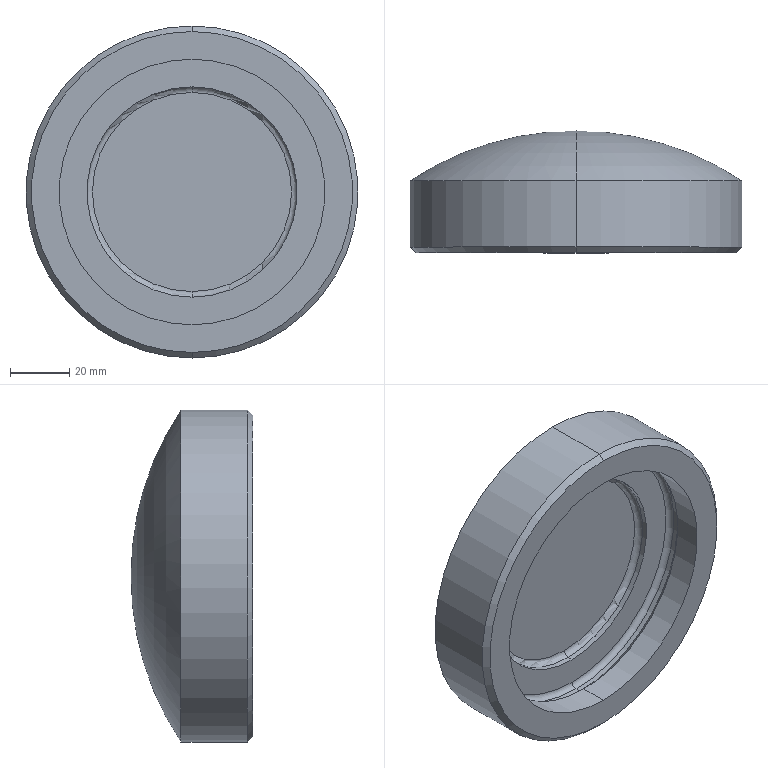Part | SolidWorks | features Chamfer 1, Revolution 1, Scale 1 | 1 solid | 21 faces | box 112.5 x 41.25 x 112.5 mm | volume 215843 mm3 | cylinder 8 | torus 6 | cone 4 | plane 3 | commonest cylinder face diameters 71.25 x2 90 x2 93.75 x2 112.5 x2
STEP:
#1=CARTESIAN_POINT('',(0.,-0.5012,-45.));
#2=VERTEX_POINT('',#1);
#3=CARTESIAN_POINT('',(0.,-0.5012,45.));
#4=VERTEX_POINT('',#3);
#5=CARTESIAN_POINT('',(0.,-0.5012,0.));
#6=DIRECTION('',(0.,1.,0.));
#7=DIRECTION('',(0.,0.,1.));
#8=AXIS2_PLACEMENT_3D('',#5,#6,#7);
#9=CIRCLE('',#8,45.);
#10=EDGE_CURVE('',#2,#4,#9,.T.);
#11=ORIENTED_EDGE('',*,*,#10,.F.);
#12=CARTESIAN_POINT('',(0.,1.374,-46.875));
#13=VERTEX_POINT('',#12);
#14=CARTESIAN_POINT('',(0.,1.374,-46.875));
#15=DIRECTION('',(0.,0.7071,-0.7071));
#16=VECTOR('',#15,1000.);
#17=LINE('',#14,#16);
#18=EDGE_CURVE('',#2,#13,#17,.T.);
#19=ORIENTED_EDGE('',*,*,#18,.T.);
#20=CARTESIAN_POINT('',(0.,1.374,46.875));
#21=VERTEX_POINT('',#20);
#22=CARTESIAN_POINT('',(0.,1.374,0.));
#23=DIRECTION('',(0.,-1.,0.));
#24=DIRECTION('',(0.,0.,-1.));
#25=AXIS2_PLACEMENT_3D('',#22,#23,#24);
#26=CIRCLE('',#25,46.875);
#27=EDGE_CURVE('',#21,#13,#26,.T.);
#28=ORIENTED_EDGE('',*,*,#27,.F.);
#29=CARTESIAN_POINT('',(0.,1.374,46.875));
#30=DIRECTION('',(0.,0.7071,0.7071));
#31=VECTOR('',#30,1000.);
#32=LINE('',#29,#31);
#33=EDGE_CURVE('',#4,#21,#32,.T.);
#34=ORIENTED_EDGE('',*,*,#33,.F.);
#35=EDGE_LOOP('',(#11,#19,#28,#34));
#36=FACE_OUTER_BOUND('',#35,.T.);
#37=CARTESIAN_POINT('',(0.,1.374,0.));
#38=DIRECTION('',(0.,1.,0.));
#39=DIRECTION('',(0.,0.,1.));
#40=AXIS2_PLACEMENT_3D('',#37,#38,#39);
#41=CONICAL_SURFACE('',#40,46.875,0.7854);
#42=ADVANCED_FACE('',(#36),#41,.F.);
#43=CARTESIAN_POINT('',(0.,3.249,46.875));
#44=VERTEX_POINT('',#43);
#45=CARTESIAN_POINT('',(0.,3.249,-46.875));
#46=VERTEX_POINT('',#45);
#47=CARTESIAN_POINT('',(0.,3.249,0.));
#48=DIRECTION('',(0.,-1.,0.));
#49=DIRECTION('',(0.,0.,-1.));
#50=AXIS2_PLACEMENT_3D('',#47,#48,#49);
#51=CIRCLE('',#50,46.875);
#52=EDGE_CURVE('',#44,#46,#51,.T.);
#53=ORIENTED_EDGE('',*,*,#52,.F.);
#54=CARTESIAN_POINT('',(0.,-9.876,46.875));
#55=DIRECTION('',(0.,-1.,0.));
#56=VECTOR('',#55,1000.);
#57=LINE('',#54,#56);
#58=EDGE_CURVE('',#44,#21,#57,.T.);
#59=ORIENTED_EDGE('',*,*,#58,.T.);
#60=ORIENTED_EDGE('',*,*,#27,.T.);
#61=CARTESIAN_POINT('',(0.,-9.876,-46.875));
#62=DIRECTION('',(0.,-1.,0.));
#63=VECTOR('',#62,1000.);
#64=LINE('',#61,#63);
#65=EDGE_CURVE('',#46,#13,#64,.T.);
#66=ORIENTED_EDGE('',*,*,#65,.F.);
#67=EDGE_LOOP('',(#53,#59,#60,#66));
#68=FACE_OUTER_BOUND('',#67,.T.);
#69=CARTESIAN_POINT('',(0.,-9.876,0.));
#70=DIRECTION('',(0.,-1.,0.));
#71=DIRECTION('',(0.,0.,-1.));
#72=AXIS2_PLACEMENT_3D('',#69,#70,#71);
#73=CYLINDRICAL_SURFACE('',#72,46.875);
#74=ADVANCED_FACE('',(#68),#73,.F.);
#75=CARTESIAN_POINT('',(0.,5.124,45.));
#76=VERTEX_POINT('',#75);
#77=CARTESIAN_POINT('',(0.,5.124,-45.));
#78=VERTEX_POINT('',#77);
#79=CARTESIAN_POINT('',(0.,5.124,0.));
#80=DIRECTION('',(0.,-1.,0.));
#81=DIRECTION('',(0.,0.,-1.));
#82=AXIS2_PLACEMENT_3D('',#79,#80,#81);
#83=CIRCLE('',#82,45.);
#84=EDGE_CURVE('',#76,#78,#83,.T.);
#85=ORIENTED_EDGE('',*,*,#84,.F.);
#86=CARTESIAN_POINT('',(0.,3.249,45.));
#87=DIRECTION('',(1.,0.,0.));
#88=DIRECTION('',(0.,0.,-1.));
#89=AXIS2_PLACEMENT_3D('',#86,#87,#88);
#90=CIRCLE('',#89,1.875);
#91=EDGE_CURVE('',#76,#44,#90,.T.);
#92=ORIENTED_EDGE('',*,*,#91,.T.);
#93=ORIENTED_EDGE('',*,*,#52,.T.);
#94=CARTESIAN_POINT('',(0.,3.249,-45.));
#95=DIRECTION('',(-1.,0.,0.));
#96=DIRECTION('',(0.,0.,1.));
#97=AXIS2_PLACEMENT_3D('',#94,#95,#96);
#98=CIRCLE('',#97,1.875);
#99=EDGE_CURVE('',#78,#46,#98,.T.);
#100=ORIENTED_EDGE('',*,*,#99,.F.);
#101=EDGE_LOOP('',(#85,#92,#93,#100));
#102=FACE_OUTER_BOUND('',#101,.T.);
#103=CARTESIAN_POINT('',(0.,3.249,0.));
#104=DIRECTION('',(0.,-1.,0.));
#105=DIRECTION('',(0.,0.,-1.));
#106=AXIS2_PLACEMENT_3D('',#103,#104,#105);
#107=TOROIDAL_SURFACE('',#106,45.,1.875);
#108=ADVANCED_FACE('',(#102),#107,.F.);
#109=CARTESIAN_POINT('',(0.,6.999,35.625));
#110=VERTEX_POINT('',#109);
#111=CARTESIAN_POINT('',(0.,6.999,-35.625));
#112=VERTEX_POINT('',#111);
#113=CARTESIAN_POINT('',(0.,6.999,0.));
#114=DIRECTION('',(0.,-1.,0.));
#115=DIRECTION('',(0.,0.,-1.));
#116=AXIS2_PLACEMENT_3D('',#113,#114,#115);
#117=CIRCLE('',#116,35.625);
#118=EDGE_CURVE('',#110,#112,#117,.T.);
#119=ORIENTED_EDGE('',*,*,#118,.F.);
#120=CARTESIAN_POINT('',(0.,5.124,35.625));
#121=VERTEX_POINT('',#120);
#122=CARTESIAN_POINT('',(0.,-9.876,35.625));
#123=DIRECTION('',(0.,-1.,0.));
#124=VECTOR('',#123,1000.);
#125=LINE('',#122,#124);
#126=EDGE_CURVE('',#110,#121,#125,.T.);
#127=ORIENTED_EDGE('',*,*,#126,.T.);
#128=CARTESIAN_POINT('',(0.,5.124,-35.625));
#129=VERTEX_POINT('',#128);
#130=CARTESIAN_POINT('',(0.,5.124,0.));
#131=DIRECTION('',(0.,-1.,0.));
#132=DIRECTION('',(0.,0.,-1.));
#133=AXIS2_PLACEMENT_3D('',#130,#131,#132);
#134=CIRCLE('',#133,35.625);
#135=EDGE_CURVE('',#121,#129,#134,.T.);
#136=ORIENTED_EDGE('',*,*,#135,.T.);
#137=CARTESIAN_POINT('',(0.,-9.876,-35.625));
#138=DIRECTION('',(0.,-1.,0.));
#139=VECTOR('',#138,1000.);
#140=LINE('',#137,#139);
#141=EDGE_CURVE('',#112,#129,#140,.T.);
#142=ORIENTED_EDGE('',*,*,#141,.F.);
#143=EDGE_LOOP('',(#119,#127,#136,#142));
#144=FACE_OUTER_BOUND('',#143,.T.);
#145=CARTESIAN_POINT('',(0.,-9.876,0.));
#146=DIRECTION('',(0.,-1.,0.));
#147=DIRECTION('',(0.,0.,-1.));
#148=AXIS2_PLACEMENT_3D('',#145,#146,#147);
#149=CYLINDRICAL_SURFACE('',#148,35.625);
#150=ADVANCED_FACE('',(#144),#149,.F.);
#151=CARTESIAN_POINT('',(0.,8.874,33.75));
#152=VERTEX_POINT('',#151);
#153=CARTESIAN_POINT('',(0.,8.874,-33.75));
#154=VERTEX_POINT('',#153);
#155=CARTESIAN_POINT('',(0.,8.874,0.));
#156=DIRECTION('',(0.,-1.,0.));
#157=DIRECTION('',(0.,0.,-1.));
#158=AXIS2_PLACEMENT_3D('',#155,#156,#157);
#159=CIRCLE('',#158,33.75);
#160=EDGE_CURVE('',#152,#154,#159,.T.);
#161=ORIENTED_EDGE('',*,*,#160,.F.);
#162=CARTESIAN_POINT('',(0.,6.999,33.75));
#163=DIRECTION('',(1.,0.,0.));
#164=DIRECTION('',(0.,0.,-1.));
#165=AXIS2_PLACEMENT_3D('',#162,#163,#164);
#166=CIRCLE('',#165,1.875);
#167=EDGE_CURVE('',#152,#110,#166,.T.);
#168=ORIENTED_EDGE('',*,*,#167,.T.);
#169=ORIENTED_EDGE('',*,*,#118,.T.);
#170=CARTESIAN_POINT('',(0.,6.999,-33.75));
#171=DIRECTION('',(-1.,0.,0.));
#172=DIRECTION('',(0.,0.,1.));
#173=AXIS2_PLACEMENT_3D('',#170,#171,#172);
#174=CIRCLE('',#173,1.875);
#175=EDGE_CURVE('',#154,#112,#174,.T.);
#176=ORIENTED_EDGE('',*,*,#175,.F.);
#177=EDGE_LOOP('',(#161,#168,#169,#176));
#178=FACE_OUTER_BOUND('',#177,.T.);
#179=CARTESIAN_POINT('',(0.,6.999,0.));
#180=DIRECTION('',(0.,-1.,0.));
#181=DIRECTION('',(0.,0.,-1.));
#182=AXIS2_PLACEMENT_3D('',#179,#180,#181);
#183=TOROIDAL_SURFACE('',#182,33.75,1.875);
#184=ADVANCED_FACE('',(#178),#183,.F.);
#185=CARTESIAN_POINT('',(0.,31.374,0.));
#186=VERTEX_POINT('',#185);
#187=CARTESIAN_POINT('',(0.,14.499,-56.25));
#188=VERTEX_POINT('',#187);
#189=CARTESIAN_POINT('',(0.,-69.876,-0.2814));
#190=DIRECTION('',(-1.,0.,0.));
#191=DIRECTION('',(0.,0.,1.));
#192=AXIS2_PLACEMENT_3D('',#189,#190,#191);
#193=CIRCLE('',#192,101.25);
#194=EDGE_CURVE('',#186,#188,#193,.T.);
#195=ORIENTED_EDGE('',*,*,#194,.F.);
#196=CARTESIAN_POINT('',(0.,14.499,56.25));
#197=VERTEX_POINT('',#196);
#198=CARTESIAN_POINT('',(0.,-69.876,0.2814));
#199=DIRECTION('',(1.,0.,0.));
#200=DIRECTION('',(0.,0.,-1.));
#201=AXIS2_PLACEMENT_3D('',#198,#199,#200);
#202=CIRCLE('',#201,101.25);
#203=EDGE_CURVE('',#186,#197,#202,.T.);
#204=ORIENTED_EDGE('',*,*,#203,.T.);
#205=CARTESIAN_POINT('',(0.,14.499,0.));
#206=DIRECTION('',(0.,-1.,0.));
#207=DIRECTION('',(0.,0.,-1.));
#208=AXIS2_PLACEMENT_3D('',#205,#206,#207);
#209=CIRCLE('',#208,56.25);
#210=EDGE_CURVE('',#188,#197,#209,.T.);
#211=ORIENTED_EDGE('',*,*,#210,.F.);
#212=EDGE_LOOP('',(#195,#204,#211));
#213=FACE_OUTER_BOUND('',#212,.T.);
#214=CARTESIAN_POINT('',(0.,-69.876,0.));
#215=DIRECTION('',(0.,-1.,0.));
#216=DIRECTION('',(0.,0.,-1.));
#217=AXIS2_PLACEMENT_3D('',#214,#215,#216);
#218=TOROIDAL_SURFACE('',#217,0.2814,101.25);
#219=ADVANCED_FACE('',(#213),#218,.T.);
#220=ORIENTED_EDGE('',*,*,#210,.T.);
#221=CARTESIAN_POINT('',(0.,-8.001,56.25));
#222=VERTEX_POINT('',#221);
#223=CARTESIAN_POINT('',(0.,-9.876,56.25));
#224=DIRECTION('',(0.,-1.,0.));
#225=VECTOR('',#224,1000.);
#226=LINE('',#223,#225);
#227=EDGE_CURVE('',#197,#222,#226,.T.);
#228=ORIENTED_EDGE('',*,*,#227,.T.);
#229=CARTESIAN_POINT('',(0.,-8.001,-56.25));
#230=VERTEX_POINT('',#229);
#231=CARTESIAN_POINT('',(0.,-8.001,0.));
#232=DIRECTION('',(0.,-1.,0.));
#233=DIRECTION('',(0.,0.,-1.));
#234=AXIS2_PLACEMENT_3D('',#231,#232,#233);
#235=CIRCLE('',#234,56.25);
#236=EDGE_CURVE('',#230,#222,#235,.T.);
#237=ORIENTED_EDGE('',*,*,#236,.F.);
#238=CARTESIAN_POINT('',(0.,-9.876,-56.25));
#239=DIRECTION('',(0.,-1.,0.));
#240=VECTOR('',#239,1000.);
#241=LINE('',#238,#240);
#242=EDGE_CURVE('',#188,#230,#241,.T.);
#243=ORIENTED_EDGE('',*,*,#242,.F.);
#244=EDGE_LOOP('',(#220,#228,#237,#243));
#245=FACE_OUTER_BOUND('',#244,.T.);
#246=CARTESIAN_POINT('',(0.,-9.876,0.));
#247=DIRECTION('',(0.,-1.,0.));
#248=DIRECTION('',(0.,0.,-1.));
#249=AXIS2_PLACEMENT_3D('',#246,#247,#248);
#250=CYLINDRICAL_SURFACE('',#249,56.25);
#251=ADVANCED_FACE('',(#245),#250,.T.);
#252=CARTESIAN_POINT('',(0.,-9.876,-54.375));
#253=VERTEX_POINT('',#252);
#254=CARTESIAN_POINT('',(0.,-9.876,54.375));
#255=VERTEX_POINT('',#254);
#256=CARTESIAN_POINT('',(0.,-9.876,0.));
#257=DIRECTION('',(0.,-1.,0.));
#258=DIRECTION('',(0.,0.,-1.));
#259=AXIS2_PLACEMENT_3D('',#256,#257,#258);
#260=CIRCLE('',#259,54.375);
#261=EDGE_CURVE('',#253,#255,#260,.T.);
#262=ORIENTED_EDGE('',*,*,#261,.F.);
#263=CARTESIAN_POINT('',(0.,-9.876,-54.375));
#264=DIRECTION('',(0.,0.7071,-0.7071));
#265=VECTOR('',#264,1000.);
#266=LINE('',#263,#265);
#267=EDGE_CURVE('',#253,#230,#266,.T.);
#268=ORIENTED_EDGE('',*,*,#267,.T.);
#269=ORIENTED_EDGE('',*,*,#236,.T.);
#270=CARTESIAN_POINT('',(0.,-9.876,54.375));
#271=DIRECTION('',(0.,0.7071,0.7071));
#272=VECTOR('',#271,1000.);
#273=LINE('',#270,#272);
#274=EDGE_CURVE('',#255,#222,#273,.T.);
#275=ORIENTED_EDGE('',*,*,#274,.F.);
#276=EDGE_LOOP('',(#262,#268,#269,#275));
#277=FACE_OUTER_BOUND('',#276,.T.);
#278=CARTESIAN_POINT('',(0.,-9.876,0.));
#279=DIRECTION('',(0.,1.,0.));
#280=DIRECTION('',(0.,0.,1.));
#281=AXIS2_PLACEMENT_3D('',#278,#279,#280);
#282=CONICAL_SURFACE('',#281,54.375,0.7854);
#283=ADVANCED_FACE('',(#277),#282,.T.);
#284=ORIENTED_EDGE('',*,*,#10,.T.);
#285=CARTESIAN_POINT('',(0.,-9.876,45.));
#286=VERTEX_POINT('',#285);
#287=CARTESIAN_POINT('',(0.,-9.876,45.));
#288=DIRECTION('',(0.,-1.,0.));
#289=VECTOR('',#288,1000.);
#290=LINE('',#287,#289);
#291=EDGE_CURVE('',#4,#286,#290,.T.);
#292=ORIENTED_EDGE('',*,*,#291,.T.);
#293=CARTESIAN_POINT('',(0.,-9.876,-45.));
#294=VERTEX_POINT('',#293);
#295=CARTESIAN_POINT('',(0.,-9.876,0.));
#296=DIRECTION('',(0.,-1.,0.));
#297=DIRECTION('',(0.,0.,-1.));
#298=AXIS2_PLACEMENT_3D('',#295,#296,#297);
#299=CIRCLE('',#298,45.);
#300=EDGE_CURVE('',#286,#294,#299,.T.);
#301=ORIENTED_EDGE('',*,*,#300,.T.);
#302=CARTESIAN_POINT('',(0.,-9.876,-45.));
#303=DIRECTION('',(0.,-1.,0.));
#304=VECTOR('',#303,1000.);
#305=LINE('',#302,#304);
#306=EDGE_CURVE('',#2,#294,#305,.T.);
#307=ORIENTED_EDGE('',*,*,#306,.F.);
#308=EDGE_LOOP('',(#284,#292,#301,#307));
#309=FACE_OUTER_BOUND('',#308,.T.);
#310=CARTESIAN_POINT('',(0.,-9.876,0.));
#311=DIRECTION('',(0.,-1.,0.));
#312=DIRECTION('',(0.,0.,-1.));
#313=AXIS2_PLACEMENT_3D('',#310,#311,#312);
#314=CYLINDRICAL_SURFACE('',#313,45.);
#315=ADVANCED_FACE('',(#309),#314,.F.);
#316=ORIENTED_EDGE('',*,*,#291,.F.);
#317=CARTESIAN_POINT('',(0.,-0.5012,0.));
#318=DIRECTION('',(0.,1.,0.));
#319=DIRECTION('',(0.,0.,1.));
#320=AXIS2_PLACEMENT_3D('',#317,#318,#319);
#321=CIRCLE('',#320,45.);
#322=EDGE_CURVE('',#4,#2,#321,.T.);
#323=ORIENTED_EDGE('',*,*,#322,.T.);
#324=ORIENTED_EDGE('',*,*,#306,.T.);
#325=CARTESIAN_POINT('',(0.,-9.876,0.));
#326=DIRECTION('',(0.,-1.,0.));
#327=DIRECTION('',(0.,0.,-1.));
#328=AXIS2_PLACEMENT_3D('',#325,#326,#327);
#329=CIRCLE('',#328,45.);
#330=EDGE_CURVE('',#294,#286,#329,.T.);
#331=ORIENTED_EDGE('',*,*,#330,.T.);
#332=EDGE_LOOP('',(#316,#323,#324,#331));
#333=FACE_OUTER_BOUND('',#332,.T.);
#334=CARTESIAN_POINT('',(0.,-9.876,0.));
#335=DIRECTION('',(0.,-1.,0.));
#336=DIRECTION('',(0.,0.,-1.));
#337=AXIS2_PLACEMENT_3D('',#334,#335,#336);
#338=CYLINDRICAL_SURFACE('',#337,45.);
#339=ADVANCED_FACE('',(#333),#338,.F.);
#340=CARTESIAN_POINT('',(0.,-9.876,0.));
#341=DIRECTION('',(0.,-1.,0.));
#342=DIRECTION('',(0.,0.,-1.));
#343=AXIS2_PLACEMENT_3D('',#340,#341,#342);
#344=CIRCLE('',#343,54.375);
#345=EDGE_CURVE('',#255,#253,#344,.T.);
#346=ORIENTED_EDGE('',*,*,#345,.T.);
#347=ORIENTED_EDGE('',*,*,#261,.T.);
#348=EDGE_LOOP('',(#346,#347));
#349=FACE_OUTER_BOUND('',#348,.T.);
#350=ORIENTED_EDGE('',*,*,#330,.F.);
#351=ORIENTED_EDGE('',*,*,#300,.F.);
#352=EDGE_LOOP('',(#350,#351));
#353=FACE_BOUND('',#352,.T.);
#354=CARTESIAN_POINT('',(45.,-9.876,0.));
#355=DIRECTION('',(0.,-1.,0.));
#356=DIRECTION('',(0.,0.,-1.));
#357=AXIS2_PLACEMENT_3D('',#354,#355,#356);
#358=PLANE('',#357);
#359=ADVANCED_FACE('',(#349,#353),#358,.T.);
#360=ORIENTED_EDGE('',*,*,#267,.F.);
#361=ORIENTED_EDGE('',*,*,#345,.F.);
#362=ORIENTED_EDGE('',*,*,#274,.T.);
#363=CARTESIAN_POINT('',(0.,-8.001,0.));
#364=DIRECTION('',(0.,-1.,0.));
#365=DIRECTION('',(0.,0.,-1.));
#366=AXIS2_PLACEMENT_3D('',#363,#364,#365);
#367=CIRCLE('',#366,56.25);
#368=EDGE_CURVE('',#222,#230,#367,.T.);
#369=ORIENTED_EDGE('',*,*,#368,.T.);
#370=EDGE_LOOP('',(#360,#361,#362,#369));
#371=FACE_OUTER_BOUND('',#370,.T.);
#372=CARTESIAN_POINT('',(0.,-9.876,0.));
#373=DIRECTION('',(0.,1.,0.));
#374=DIRECTION('',(0.,0.,1.));
#375=AXIS2_PLACEMENT_3D('',#372,#373,#374);
#376=CONICAL_SURFACE('',#375,54.375,0.7854);
#377=ADVANCED_FACE('',(#371),#376,.T.);
#378=ORIENTED_EDGE('',*,*,#227,.F.);
#379=CARTESIAN_POINT('',(0.,14.499,0.));
#380=DIRECTION('',(0.,-1.,0.));
#381=DIRECTION('',(0.,0.,-1.));
#382=AXIS2_PLACEMENT_3D('',#379,#380,#381);
#383=CIRCLE('',#382,56.25);
#384=EDGE_CURVE('',#197,#188,#383,.T.);
#385=ORIENTED_EDGE('',*,*,#384,.T.);
#386=ORIENTED_EDGE('',*,*,#242,.T.);
#387=ORIENTED_EDGE('',*,*,#368,.F.);
#388=EDGE_LOOP('',(#378,#385,#386,#387));
#389=FACE_OUTER_BOUND('',#388,.T.);
#390=CARTESIAN_POINT('',(0.,-9.876,0.));
#391=DIRECTION('',(0.,-1.,0.));
#392=DIRECTION('',(0.,0.,-1.));
#393=AXIS2_PLACEMENT_3D('',#390,#391,#392);
#394=CYLINDRICAL_SURFACE('',#393,56.25);
#395=ADVANCED_FACE('',(#389),#394,.T.);
#396=ORIENTED_EDGE('',*,*,#203,.F.);
#397=ORIENTED_EDGE('',*,*,#194,.T.);
#398=ORIENTED_EDGE('',*,*,#384,.F.);
#399=EDGE_LOOP('',(#396,#397,#398));
#400=FACE_OUTER_BOUND('',#399,.T.);
#401=CARTESIAN_POINT('',(0.,-69.876,0.));
#402=DIRECTION('',(0.,-1.,0.));
#403=DIRECTION('',(0.,0.,-1.));
#404=AXIS2_PLACEMENT_3D('',#401,#402,#403);
#405=TOROIDAL_SURFACE('',#404,0.2814,101.25);
#406=ADVANCED_FACE('',(#400),#405,.T.);
#407=CARTESIAN_POINT('',(0.,8.874,0.));
#408=DIRECTION('',(0.,-1.,0.));
#409=DIRECTION('',(0.,0.,-1.));
#410=AXIS2_PLACEMENT_3D('',#407,#408,#409);
#411=CIRCLE('',#410,33.75);
#412=EDGE_CURVE('',#154,#152,#411,.T.);
#413=ORIENTED_EDGE('',*,*,#412,.T.);
#414=ORIENTED_EDGE('',*,*,#160,.T.);
#415=EDGE_LOOP('',(#413,#414));
#416=FACE_OUTER_BOUND('',#415,.T.);
#417=CARTESIAN_POINT('',(33.75,8.874,0.));
#418=DIRECTION('',(0.,-1.,0.));
#419=DIRECTION('',(0.,0.,-1.));
#420=AXIS2_PLACEMENT_3D('',#417,#418,#419);
#421=PLANE('',#420);
#422=ADVANCED_FACE('',(#416),#421,.T.);
#423=ORIENTED_EDGE('',*,*,#167,.F.);
#424=ORIENTED_EDGE('',*,*,#412,.F.);
#425=ORIENTED_EDGE('',*,*,#175,.T.);
#426=CARTESIAN_POINT('',(0.,6.999,0.));
#427=DIRECTION('',(0.,-1.,0.));
#428=DIRECTION('',(0.,0.,-1.));
#429=AXIS2_PLACEMENT_3D('',#426,#427,#428);
#430=CIRCLE('',#429,35.625);
#431=EDGE_CURVE('',#112,#110,#430,.T.);
#432=ORIENTED_EDGE('',*,*,#431,.T.);
#433=EDGE_LOOP('',(#423,#424,#425,#432));
#434=FACE_OUTER_BOUND('',#433,.T.);
#435=CARTESIAN_POINT('',(0.,6.999,0.));
#436=DIRECTION('',(0.,-1.,0.));
#437=DIRECTION('',(0.,0.,-1.));
#438=AXIS2_PLACEMENT_3D('',#435,#436,#437);
#439=TOROIDAL_SURFACE('',#438,33.75,1.875);
#440=ADVANCED_FACE('',(#434),#439,.F.);
#441=ORIENTED_EDGE('',*,*,#126,.F.);
#442=ORIENTED_EDGE('',*,*,#431,.F.);
#443=ORIENTED_EDGE('',*,*,#141,.T.);
#444=CARTESIAN_POINT('',(0.,5.124,0.));
#445=DIRECTION('',(0.,-1.,0.));
#446=DIRECTION('',(0.,0.,-1.));
#447=AXIS2_PLACEMENT_3D('',#444,#445,#446);
#448=CIRCLE('',#447,35.625);
#449=EDGE_CURVE('',#129,#121,#448,.T.);
#450=ORIENTED_EDGE('',*,*,#449,.T.);
#451=EDGE_LOOP('',(#441,#442,#443,#450));
#452=FACE_OUTER_BOUND('',#451,.T.);
#453=CARTESIAN_POINT('',(0.,-9.876,0.));
#454=DIRECTION('',(0.,-1.,0.));
#455=DIRECTION('',(0.,0.,-1.));
#456=AXIS2_PLACEMENT_3D('',#453,#454,#455);
#457=CYLINDRICAL_SURFACE('',#456,35.625);
#458=ADVANCED_FACE('',(#452),#457,.F.);
#459=CARTESIAN_POINT('',(0.,5.124,0.));
#460=DIRECTION('',(0.,-1.,0.));
#461=DIRECTION('',(0.,0.,-1.));
#462=AXIS2_PLACEMENT_3D('',#459,#460,#461);
#463=CIRCLE('',#462,45.);
#464=EDGE_CURVE('',#78,#76,#463,.T.);
#465=ORIENTED_EDGE('',*,*,#464,.T.);
#466=ORIENTED_EDGE('',*,*,#84,.T.);
#467=EDGE_LOOP('',(#465,#466));
#468=FACE_OUTER_BOUND('',#467,.T.);
#469=ORIENTED_EDGE('',*,*,#449,.F.);
#470=ORIENTED_EDGE('',*,*,#135,.F.);
#471=EDGE_LOOP('',(#469,#470));
#472=FACE_BOUND('',#471,.T.);
#473=CARTESIAN_POINT('',(45.,5.124,0.));
#474=DIRECTION('',(0.,-1.,0.));
#475=DIRECTION('',(0.,0.,-1.));
#476=AXIS2_PLACEMENT_3D('',#473,#474,#475);
#477=PLANE('',#476);
#478=ADVANCED_FACE('',(#468,#472),#477,.T.);
#479=ORIENTED_EDGE('',*,*,#91,.F.);
#480=ORIENTED_EDGE('',*,*,#464,.F.);
#481=ORIENTED_EDGE('',*,*,#99,.T.);
#482=CARTESIAN_POINT('',(0.,3.249,0.));
#483=DIRECTION('',(0.,-1.,0.));
#484=DIRECTION('',(0.,0.,-1.));
#485=AXIS2_PLACEMENT_3D('',#482,#483,#484);
#486=CIRCLE('',#485,46.875);
#487=EDGE_CURVE('',#46,#44,#486,.T.);
#488=ORIENTED_EDGE('',*,*,#487,.T.);
#489=EDGE_LOOP('',(#479,#480,#481,#488));
#490=FACE_OUTER_BOUND('',#489,.T.);
#491=CARTESIAN_POINT('',(0.,3.249,0.));
#492=DIRECTION('',(0.,-1.,0.));
#493=DIRECTION('',(0.,0.,-1.));
#494=AXIS2_PLACEMENT_3D('',#491,#492,#493);
#495=TOROIDAL_SURFACE('',#494,45.,1.875);
#496=ADVANCED_FACE('',(#490),#495,.F.);
#497=ORIENTED_EDGE('',*,*,#58,.F.);
#498=ORIENTED_EDGE('',*,*,#487,.F.);
#499=ORIENTED_EDGE('',*,*,#65,.T.);
#500=CARTESIAN_POINT('',(0.,1.374,0.));
#501=DIRECTION('',(0.,-1.,0.));
#502=DIRECTION('',(0.,0.,-1.));
#503=AXIS2_PLACEMENT_3D('',#500,#501,#502);
#504=CIRCLE('',#503,46.875);
#505=EDGE_CURVE('',#13,#21,#504,.T.);
#506=ORIENTED_EDGE('',*,*,#505,.T.);
#507=EDGE_LOOP('',(#497,#498,#499,#506));
#508=FACE_OUTER_BOUND('',#507,.T.);
#509=CARTESIAN_POINT('',(0.,-9.876,0.));
#510=DIRECTION('',(0.,-1.,0.));
#511=DIRECTION('',(0.,0.,-1.));
#512=AXIS2_PLACEMENT_3D('',#509,#510,#511);
#513=CYLINDRICAL_SURFACE('',#512,46.875);
#514=ADVANCED_FACE('',(#508),#513,.F.);
#515=ORIENTED_EDGE('',*,*,#18,.F.);
#516=ORIENTED_EDGE('',*,*,#322,.F.);
#517=ORIENTED_EDGE('',*,*,#33,.T.);
#518=ORIENTED_EDGE('',*,*,#505,.F.);
#519=EDGE_LOOP('',(#515,#516,#517,#518));
#520=FACE_OUTER_BOUND('',#519,.T.);
#521=CARTESIAN_POINT('',(0.,1.374,0.));
#522=DIRECTION('',(0.,1.,0.));
#523=DIRECTION('',(0.,0.,1.));
#524=AXIS2_PLACEMENT_3D('',#521,#522,#523);
#525=CONICAL_SURFACE('',#524,46.875,0.7854);
#526=ADVANCED_FACE('',(#520),#525,.F.);
#527=CLOSED_SHELL('',(#42,#74,#108,#150,#184,#219,#251,#283,#315,#339,#359,#377,#395,#406,#422,#440,#458,#478,#496,#514,#526));
#528=MANIFOLD_SOLID_BREP('',#527);
#529=CARTESIAN_POINT('',(0.,0.,0.));
#530=DIRECTION('',(0.,0.,1.));
#531=DIRECTION('',(1.,0.,0.));
#532=AXIS2_PLACEMENT_3D('',#529,#530,#531);
#533=(LENGTH_UNIT()NAMED_UNIT(*)SI_UNIT(.MILLI.,.METRE.));
#534=UNCERTAINTY_MEASURE_WITH_UNIT(LENGTH_MEASURE(0.00001),#533,'','');
#535=(NAMED_UNIT(*)PLANE_ANGLE_UNIT()SI_UNIT($,.RADIAN.));
#536=(NAMED_UNIT(*)SI_UNIT($,.STERADIAN.)SOLID_ANGLE_UNIT());
#537=(GEOMETRIC_REPRESENTATION_CONTEXT(3)GLOBAL_UNCERTAINTY_ASSIGNED_CONTEXT((#534))GLOBAL_UNIT_ASSIGNED_CONTEXT((#533,#535,#536))REPRESENTATION_CONTEXT('',''));
#538=ADVANCED_BREP_SHAPE_REPRESENTATION('',(#528,#532),#537);